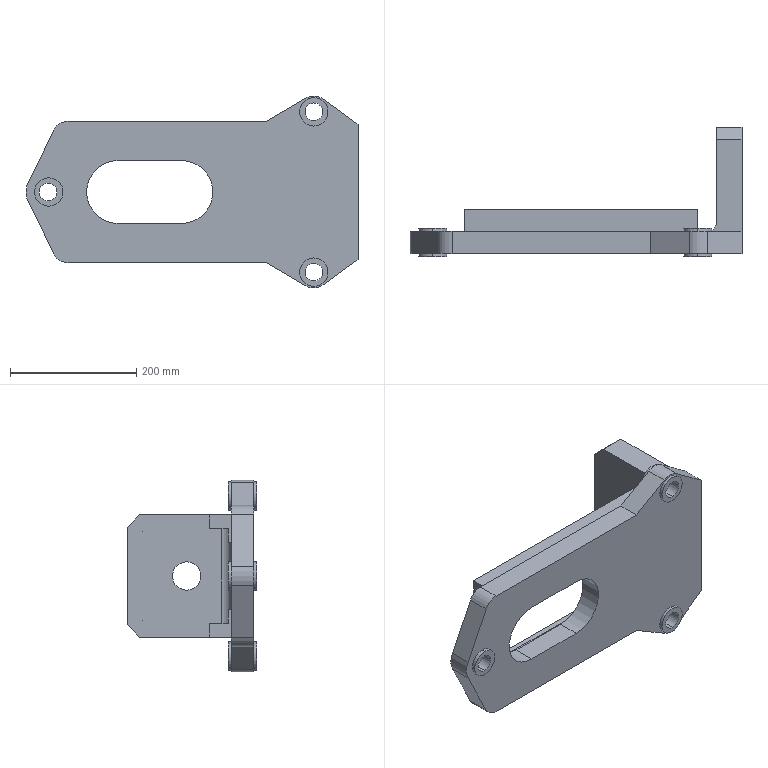Part | SolidWorks | features ICE 7, HoleWzd 3, 3DProfileFeature 1, Extrusion 1, Fillet 1, WeldmentFeature 1 | 3 solids | 151 faces | box 526.008 x 205 x 304.212 mm | volume 5277088 mm3 | cylinder 55 | cone 54 | plane 42 | commonest cylinder face diameters 8.5 x16 45 x14 16 x8 28 x6 50.212 x3 50 x2